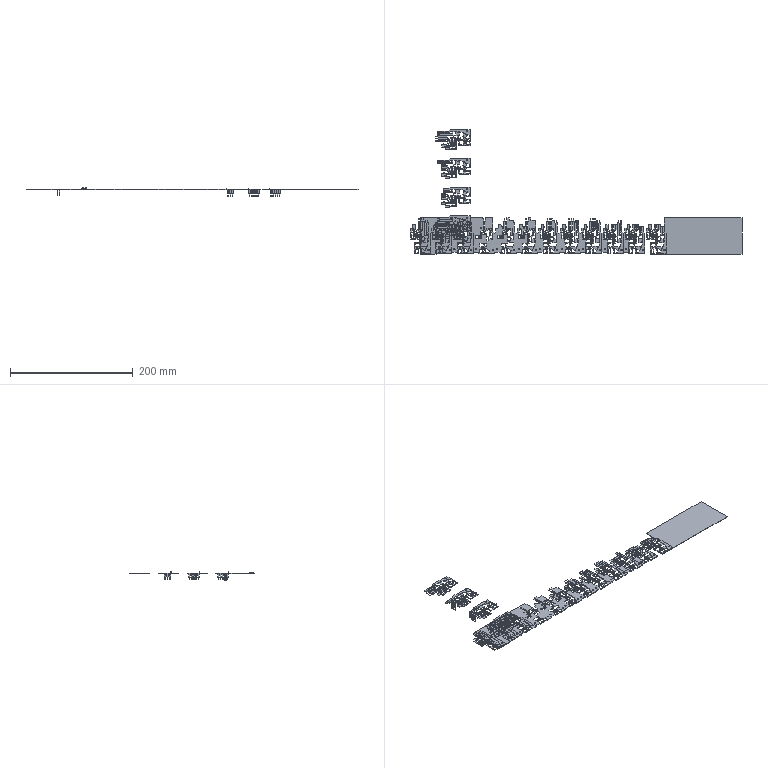Part | NX | features BREP 11 | 20 solids | 5773 faces | volume 19397 mm3 | plane 3175 | cylinder 2598 | commonest cylinder face diameters 1 x2416 2.2 x45 2 x34 72.496 x23 188.049 x22 72.701 x20